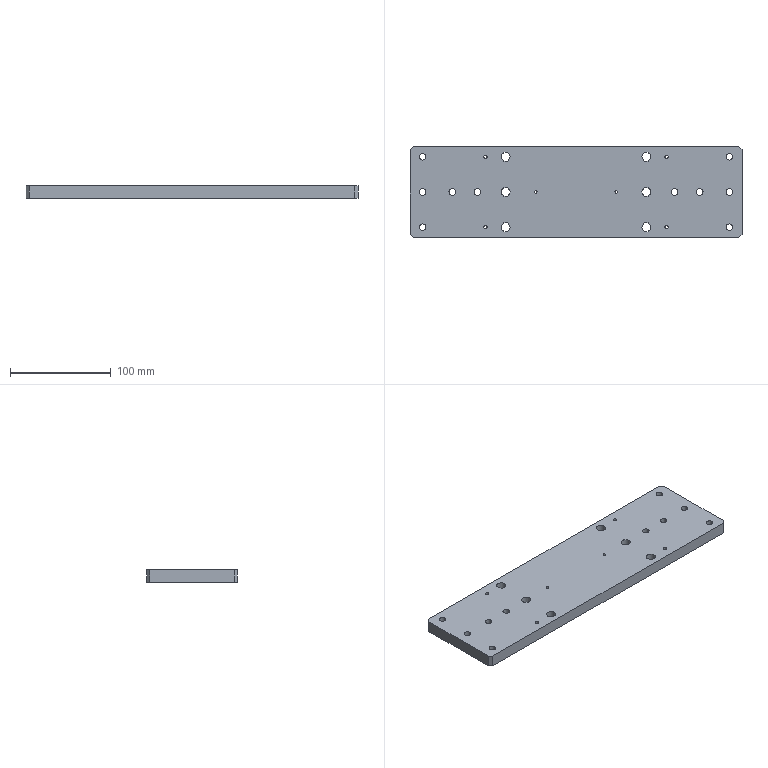CAM job | NX | 3-axis milling, drilling | part box 330 x 90 x 12 mm | stock box 335 x 100 x 15 mm
Tools:
number,name,description,diameter,corner_radius,flute_length,length,flutes
6,D6,平底铣刀-粗,6.0,0.0,25.0,75.0,2
9,D10,平底铣刀-粗,10.0,0.0,35.0,75.0,2
7,D6-J,平底铣刀-精,6.0,0.0,25.0,75.0,2
10,D10-J,平底铣刀-精,10.0,0.0,35.0,75.0,2
1,D80R0.8飞刀,圆鼻刀-粗,80.0,0.8,50.0,75.0,2
1,D80R0.8飞刀-J,圆鼻刀-精,80.0,0.8,50.0,75.0,2
2,D6倒角刀,倒角刀,6.0,0.0,3.0,25.0,2
20,M3X0.5,丝锥,2.5,0.0,35.0,50.0,2
21,M4X0.7,丝锥,3.3,0.0,35.0,50.0,2
12,ZT2.5,钻头,2.5,0.0,35.0,50.0,2
17,ZT6.6,钻头,6.6,0.0,35.0,50.0,2
18,ZT9,钻头,9.0,0.0,35.0,50.0,2
13,钻头3.3,Twist Drill 3.3 mm,3.3,0.0,35.0,35.008,2
Operations:
program,operation,operation_type,tool,method,geometry_group,spindle_rpm,surface_speed,feed_per_tooth,feed_cut,feed_plunge,cut_length_mm,path_length_mm,cut_time_min,machine_time_min
B,底壁铣飞面开粗_COPY,VolumeBased25DMillingOperation,D80R0.8飞刀,分层开粗-切深K-步距G,W-B,2800.0,703.696,0.5357,3000.0,100.0,5260.185,5467.751,1.753,1.774
B,底壁铣飞面精光_COPY,VolumeBased25DMillingOperation,D80R0.8飞刀-J,侧刃精光-切深K-步距G,W-B,4000.0,1005.28,0.125,1000.0,100.0,876.11,912.11,0.8761,0.8797
B,钻倒角_3,Operation,D6倒角刀,METHOD,W-B,8000.0,150.796,0.0625,1000.0,0.0,9.5,142.056,0.0095,0.0228
B,钻倒角_4,Operation,D6倒角刀,METHOD,W-B,8000.0,150.796,0.0625,1000.0,0.0,20.8,410.753,0.0208,0.0598
B,铣倒角_3,PlanarMilling,D6倒角刀,METHOD,W-B,8000.0,150.796,0.075,1200.0,100.0,204.46,1100.252,0.1704,0.26
B,铣倒角_4,PlanarMilling,D6倒角刀,METHOD,W-B,8000.0,150.796,0.075,1200.0,100.0,140.517,682.149,0.1171,0.1713
B,C0.3封闭铣廓倒角6X45L_COPY,PlanarMilling,D6倒角刀,爬面_倒角-切深0-步距G,W-B,7000.0,131.0,0.1071,1500.0,100.0,850.499,886.499,0.567,0.5706
A,顶面,FaceMilling,D80R0.8飞刀,侧刃精光-切深K-步距G,W-A,4000.0,1005.31,0.125,1000.0,100.0,1329.0,1365.0,1.329,1.333
A,外形粗_2,VolumeBased25DMillingOperation,D10,METHOD,W-A,8000.0,251.327,0.3125,5000.0,80.0,14706.758,14757.558,2.941,2.946
A,打点-深0.8,Operation,D6倒角刀,NONE,W-A,8000.0,150.796,0.0312,500.0,90.0,39.6,896.699,0.0792,0.1649
A,沉头孔-钻孔0段,Operation,ZT6.6,NONE,W-A,1200.0,24.881,0.0625,150.0,90.0,169.828,866.326,1.132,1.202
A,通孔-8-10,Operation,ZT9,NONE,W-A,1800.0,50.894,0.0417,150.0,90.0,106.223,537.507,0.7082,0.7513
A,通孔-M3螺纹底孔,Operation,ZT2.5,NONE,W-A,3000.0,23.562,0.05,300.0,90.0,37.502,196.011,0.125,0.1409
A,通孔-M4螺纹底孔,Operation,钻头3.3,NONE,W-A,3000.0,31.102,0.05,300.0,90.0,75.966,514.948,0.2532,0.2971
A,铣孔开粗D6_1,CylinderMilling,D6,NONE,W-A,8000.0,150.796,0.075,1200.0,100.0,2308.329,3244.877,1.924,2.017
A,铣孔精光D6_1,CylinderMilling,D6-J,精光步距切深关,W-A,8000.0,150.796,0.0312,500.0,100.0,446.153,1387.701,0.8923,0.9865
A,仅选体,SurfaceContour,D6倒角刀,METHOD,W-A,8000.0,150.796,0.1875,3000.0,100.0,850.272,886.073,0.2834,0.287
A,钻倒角_1,Operation,D6倒角刀,METHOD,W-A,8000.0,150.796,0.0312,500.0,0.0,9.5,142.056,0.019,0.0323
A,钻倒角_2,Operation,D6倒角刀,METHOD,W-A,8000.0,150.796,0.0312,500.0,0.0,20.8,410.753,0.0416,0.0806
A,铣倒角_1,PlanarMilling,D6倒角刀,METHOD,W-A,8000.0,150.796,0.05,800.0,100.0,209.463,735.568,0.2618,0.3144
A,铣倒角_2,PlanarMilling,D6倒角刀,NONE,W-A,8000.0,150.796,0.05,800.0,100.0,433.926,1292.458,0.5424,0.6283
A,通孔-攻牙M3,Operation,M3X0.5,METHOD,W-A,800.0,6.283,0.0003,0.5,90.0,32.0,185.006,64.0,64.015
A,通孔-攻牙M4,Operation,M4X0.7,METHOD,W-A,600.0,6.22,0.0006,0.7,90.0,64.0,491.017,91.429,91.471
A,外形半精_2,VolumeBased25DMillingOperation,D10-J,METHOD,W-A,8000.0,251.327,0.0625,1000.0,100.0,869.345,932.945,0.8693,0.8757